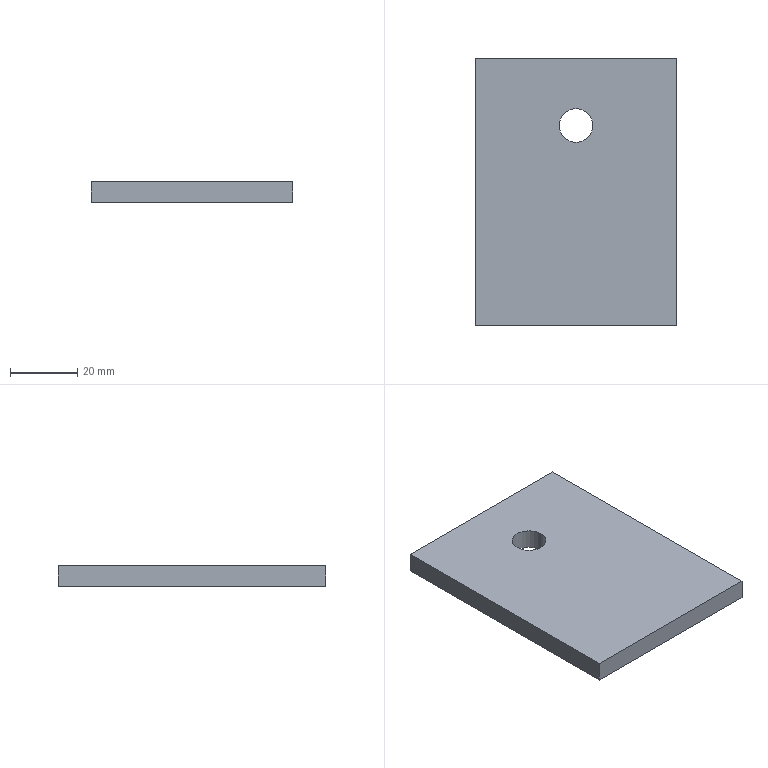Part | SolidWorks | features FlatPattern 1, SMBaseFlange 1, SheetMetal 1 | 1 solid | 8 faces | box 60 x 79.5 x 6 mm | volume 28149 mm3 | plane 6 | cylinder 2 | commonest cylinder face diameters 10 x2
STEP:
#1=CARTESIAN_POINT('',(25.,59.5,-6.));
#2=VERTEX_POINT('',#1);
#3=CARTESIAN_POINT('',(35.,59.5,-6.));
#4=VERTEX_POINT('',#3);
#5=CARTESIAN_POINT('',(30.,59.5,-6.));
#6=DIRECTION('',(0.,0.,1.));
#7=DIRECTION('',(1.,0.,0.));
#8=AXIS2_PLACEMENT_3D('',#5,#6,#7);
#9=CIRCLE('',#8,5.);
#10=EDGE_CURVE('',#2,#4,#9,.T.);
#11=ORIENTED_EDGE('',*,*,#10,.F.);
#12=CARTESIAN_POINT('',(25.,59.5,0.));
#13=VERTEX_POINT('',#12);
#14=CARTESIAN_POINT('',(25.,59.5,-6.));
#15=DIRECTION('',(0.,0.,1.));
#16=VECTOR('',#15,1000.);
#17=LINE('',#14,#16);
#18=EDGE_CURVE('',#2,#13,#17,.T.);
#19=ORIENTED_EDGE('',*,*,#18,.T.);
#20=CARTESIAN_POINT('',(35.,59.5,0.));
#21=VERTEX_POINT('',#20);
#22=CARTESIAN_POINT('',(30.,59.5,0.));
#23=DIRECTION('',(0.,0.,1.));
#24=DIRECTION('',(1.,0.,0.));
#25=AXIS2_PLACEMENT_3D('',#22,#23,#24);
#26=CIRCLE('',#25,5.);
#27=EDGE_CURVE('',#13,#21,#26,.T.);
#28=ORIENTED_EDGE('',*,*,#27,.T.);
#29=CARTESIAN_POINT('',(35.,59.5,-6.));
#30=DIRECTION('',(0.,0.,1.));
#31=VECTOR('',#30,1000.);
#32=LINE('',#29,#31);
#33=EDGE_CURVE('',#4,#21,#32,.T.);
#34=ORIENTED_EDGE('',*,*,#33,.F.);
#35=EDGE_LOOP('',(#11,#19,#28,#34));
#36=FACE_OUTER_BOUND('',#35,.T.);
#37=CARTESIAN_POINT('',(30.,59.5,-6.));
#38=DIRECTION('',(0.,0.,1.));
#39=DIRECTION('',(1.,0.,0.));
#40=AXIS2_PLACEMENT_3D('',#37,#38,#39);
#41=CYLINDRICAL_SURFACE('',#40,5.);
#42=ADVANCED_FACE('',(#36),#41,.F.);
#43=CARTESIAN_POINT('',(0.,79.5,0.));
#44=VERTEX_POINT('',#43);
#45=CARTESIAN_POINT('',(0.,0.,0.));
#46=VERTEX_POINT('',#45);
#47=CARTESIAN_POINT('',(0.,0.,0.));
#48=DIRECTION('',(0.,-1.,0.));
#49=VECTOR('',#48,1000.);
#50=LINE('',#47,#49);
#51=EDGE_CURVE('',#44,#46,#50,.T.);
#52=ORIENTED_EDGE('',*,*,#51,.F.);
#53=CARTESIAN_POINT('',(0.,79.5,-6.));
#54=VERTEX_POINT('',#53);
#55=CARTESIAN_POINT('',(0.,79.5,-6.));
#56=DIRECTION('',(0.,0.,1.));
#57=VECTOR('',#56,1000.);
#58=LINE('',#55,#57);
#59=EDGE_CURVE('',#54,#44,#58,.T.);
#60=ORIENTED_EDGE('',*,*,#59,.F.);
#61=CARTESIAN_POINT('',(0.,0.,-6.));
#62=VERTEX_POINT('',#61);
#63=CARTESIAN_POINT('',(0.,0.,-6.));
#64=DIRECTION('',(0.,-1.,0.));
#65=VECTOR('',#64,1000.);
#66=LINE('',#63,#65);
#67=EDGE_CURVE('',#54,#62,#66,.T.);
#68=ORIENTED_EDGE('',*,*,#67,.T.);
#69=CARTESIAN_POINT('',(0.,0.,-6.));
#70=DIRECTION('',(0.,0.,1.));
#71=VECTOR('',#70,1000.);
#72=LINE('',#69,#71);
#73=EDGE_CURVE('',#62,#46,#72,.T.);
#74=ORIENTED_EDGE('',*,*,#73,.T.);
#75=EDGE_LOOP('',(#52,#60,#68,#74));
#76=FACE_OUTER_BOUND('',#75,.T.);
#77=CARTESIAN_POINT('',(0.,0.,-6.));
#78=DIRECTION('',(-1.,0.,0.));
#79=DIRECTION('',(0.,0.,1.));
#80=AXIS2_PLACEMENT_3D('',#77,#78,#79);
#81=PLANE('',#80);
#82=ADVANCED_FACE('',(#76),#81,.T.);
#83=CARTESIAN_POINT('',(60.,79.5,0.));
#84=VERTEX_POINT('',#83);
#85=CARTESIAN_POINT('',(0.,79.5,0.));
#86=DIRECTION('',(-1.,0.,0.));
#87=VECTOR('',#86,1000.);
#88=LINE('',#85,#87);
#89=EDGE_CURVE('',#84,#44,#88,.T.);
#90=ORIENTED_EDGE('',*,*,#89,.F.);
#91=CARTESIAN_POINT('',(60.,79.5,-6.));
#92=VERTEX_POINT('',#91);
#93=CARTESIAN_POINT('',(60.,79.5,-6.));
#94=DIRECTION('',(0.,0.,1.));
#95=VECTOR('',#94,1000.);
#96=LINE('',#93,#95);
#97=EDGE_CURVE('',#92,#84,#96,.T.);
#98=ORIENTED_EDGE('',*,*,#97,.F.);
#99=CARTESIAN_POINT('',(0.,79.5,-6.));
#100=DIRECTION('',(-1.,0.,0.));
#101=VECTOR('',#100,1000.);
#102=LINE('',#99,#101);
#103=EDGE_CURVE('',#92,#54,#102,.T.);
#104=ORIENTED_EDGE('',*,*,#103,.T.);
#105=ORIENTED_EDGE('',*,*,#59,.T.);
#106=EDGE_LOOP('',(#90,#98,#104,#105));
#107=FACE_OUTER_BOUND('',#106,.T.);
#108=CARTESIAN_POINT('',(0.,79.5,-6.));
#109=DIRECTION('',(0.,1.,0.));
#110=DIRECTION('',(0.,0.,1.));
#111=AXIS2_PLACEMENT_3D('',#108,#109,#110);
#112=PLANE('',#111);
#113=ADVANCED_FACE('',(#107),#112,.T.);
#114=CARTESIAN_POINT('',(60.,0.,0.));
#115=VERTEX_POINT('',#114);
#116=CARTESIAN_POINT('',(60.,0.,0.));
#117=DIRECTION('',(0.,1.,0.));
#118=VECTOR('',#117,1000.);
#119=LINE('',#116,#118);
#120=EDGE_CURVE('',#115,#84,#119,.T.);
#121=ORIENTED_EDGE('',*,*,#120,.F.);
#122=CARTESIAN_POINT('',(60.,0.,-6.));
#123=VERTEX_POINT('',#122);
#124=CARTESIAN_POINT('',(60.,0.,-6.));
#125=DIRECTION('',(0.,0.,1.));
#126=VECTOR('',#125,1000.);
#127=LINE('',#124,#126);
#128=EDGE_CURVE('',#123,#115,#127,.T.);
#129=ORIENTED_EDGE('',*,*,#128,.F.);
#130=CARTESIAN_POINT('',(60.,0.,-6.));
#131=DIRECTION('',(0.,1.,0.));
#132=VECTOR('',#131,1000.);
#133=LINE('',#130,#132);
#134=EDGE_CURVE('',#123,#92,#133,.T.);
#135=ORIENTED_EDGE('',*,*,#134,.T.);
#136=ORIENTED_EDGE('',*,*,#97,.T.);
#137=EDGE_LOOP('',(#121,#129,#135,#136));
#138=FACE_OUTER_BOUND('',#137,.T.);
#139=CARTESIAN_POINT('',(60.,0.,-6.));
#140=DIRECTION('',(1.,0.,0.));
#141=DIRECTION('',(0.,0.,-1.));
#142=AXIS2_PLACEMENT_3D('',#139,#140,#141);
#143=PLANE('',#142);
#144=ADVANCED_FACE('',(#138),#143,.T.);
#145=CARTESIAN_POINT('',(0.,0.,0.));
#146=DIRECTION('',(1.,0.,0.));
#147=VECTOR('',#146,1000.);
#148=LINE('',#145,#147);
#149=EDGE_CURVE('',#46,#115,#148,.T.);
#150=ORIENTED_EDGE('',*,*,#149,.F.);
#151=ORIENTED_EDGE('',*,*,#73,.F.);
#152=CARTESIAN_POINT('',(0.,0.,-6.));
#153=DIRECTION('',(1.,0.,0.));
#154=VECTOR('',#153,1000.);
#155=LINE('',#152,#154);
#156=EDGE_CURVE('',#62,#123,#155,.T.);
#157=ORIENTED_EDGE('',*,*,#156,.T.);
#158=ORIENTED_EDGE('',*,*,#128,.T.);
#159=EDGE_LOOP('',(#150,#151,#157,#158));
#160=FACE_OUTER_BOUND('',#159,.T.);
#161=CARTESIAN_POINT('',(0.,0.,-6.));
#162=DIRECTION('',(0.,-1.,0.));
#163=DIRECTION('',(0.,0.,-1.));
#164=AXIS2_PLACEMENT_3D('',#161,#162,#163);
#165=PLANE('',#164);
#166=ADVANCED_FACE('',(#160),#165,.T.);
#167=CARTESIAN_POINT('',(30.,59.5,-6.));
#168=DIRECTION('',(0.,0.,1.));
#169=DIRECTION('',(1.,0.,0.));
#170=AXIS2_PLACEMENT_3D('',#167,#168,#169);
#171=CIRCLE('',#170,5.);
#172=EDGE_CURVE('',#4,#2,#171,.T.);
#173=ORIENTED_EDGE('',*,*,#172,.T.);
#174=ORIENTED_EDGE('',*,*,#10,.T.);
#175=EDGE_LOOP('',(#173,#174));
#176=FACE_BOUND('',#175,.T.);
#177=ORIENTED_EDGE('',*,*,#67,.F.);
#178=ORIENTED_EDGE('',*,*,#103,.F.);
#179=ORIENTED_EDGE('',*,*,#134,.F.);
#180=ORIENTED_EDGE('',*,*,#156,.F.);
#181=EDGE_LOOP('',(#177,#178,#179,#180));
#182=FACE_OUTER_BOUND('',#181,.T.);
#183=CARTESIAN_POINT('',(0.,0.,-6.));
#184=DIRECTION('',(0.,0.,-1.));
#185=DIRECTION('',(-1.,0.,0.));
#186=AXIS2_PLACEMENT_3D('',#183,#184,#185);
#187=PLANE('',#186);
#188=ADVANCED_FACE('',(#176,#182),#187,.T.);
#189=CARTESIAN_POINT('',(30.,59.5,0.));
#190=DIRECTION('',(0.,0.,1.));
#191=DIRECTION('',(1.,0.,0.));
#192=AXIS2_PLACEMENT_3D('',#189,#190,#191);
#193=CIRCLE('',#192,5.);
#194=EDGE_CURVE('',#21,#13,#193,.T.);
#195=ORIENTED_EDGE('',*,*,#194,.F.);
#196=ORIENTED_EDGE('',*,*,#27,.F.);
#197=EDGE_LOOP('',(#195,#196));
#198=FACE_BOUND('',#197,.T.);
#199=ORIENTED_EDGE('',*,*,#51,.T.);
#200=ORIENTED_EDGE('',*,*,#149,.T.);
#201=ORIENTED_EDGE('',*,*,#120,.T.);
#202=ORIENTED_EDGE('',*,*,#89,.T.);
#203=EDGE_LOOP('',(#199,#200,#201,#202));
#204=FACE_OUTER_BOUND('',#203,.T.);
#205=CARTESIAN_POINT('',(0.,0.,0.));
#206=DIRECTION('',(0.,0.,-1.));
#207=DIRECTION('',(-1.,0.,0.));
#208=AXIS2_PLACEMENT_3D('',#205,#206,#207);
#209=PLANE('',#208);
#210=ADVANCED_FACE('',(#198,#204),#209,.F.);
#211=ORIENTED_EDGE('',*,*,#18,.F.);
#212=ORIENTED_EDGE('',*,*,#172,.F.);
#213=ORIENTED_EDGE('',*,*,#33,.T.);
#214=ORIENTED_EDGE('',*,*,#194,.T.);
#215=EDGE_LOOP('',(#211,#212,#213,#214));
#216=FACE_OUTER_BOUND('',#215,.T.);
#217=CARTESIAN_POINT('',(30.,59.5,-6.));
#218=DIRECTION('',(0.,0.,1.));
#219=DIRECTION('',(1.,0.,0.));
#220=AXIS2_PLACEMENT_3D('',#217,#218,#219);
#221=CYLINDRICAL_SURFACE('',#220,5.);
#222=ADVANCED_FACE('',(#216),#221,.F.);
#223=CLOSED_SHELL('',(#42,#82,#113,#144,#166,#188,#210,#222));
#224=MANIFOLD_SOLID_BREP('',#223);
#225=CARTESIAN_POINT('',(0.,0.,0.));
#226=DIRECTION('',(0.,0.,1.));
#227=DIRECTION('',(1.,0.,0.));
#228=AXIS2_PLACEMENT_3D('',#225,#226,#227);
#229=(LENGTH_UNIT()NAMED_UNIT(*)SI_UNIT(.MILLI.,.METRE.));
#230=UNCERTAINTY_MEASURE_WITH_UNIT(LENGTH_MEASURE(0.00001),#229,'','');
#231=(NAMED_UNIT(*)PLANE_ANGLE_UNIT()SI_UNIT($,.RADIAN.));
#232=(NAMED_UNIT(*)SI_UNIT($,.STERADIAN.)SOLID_ANGLE_UNIT());
#233=(GEOMETRIC_REPRESENTATION_CONTEXT(3)GLOBAL_UNCERTAINTY_ASSIGNED_CONTEXT((#230))GLOBAL_UNIT_ASSIGNED_CONTEXT((#229,#231,#232))REPRESENTATION_CONTEXT('',''));
#234=ADVANCED_BREP_SHAPE_REPRESENTATION('',(#224,#228),#233);